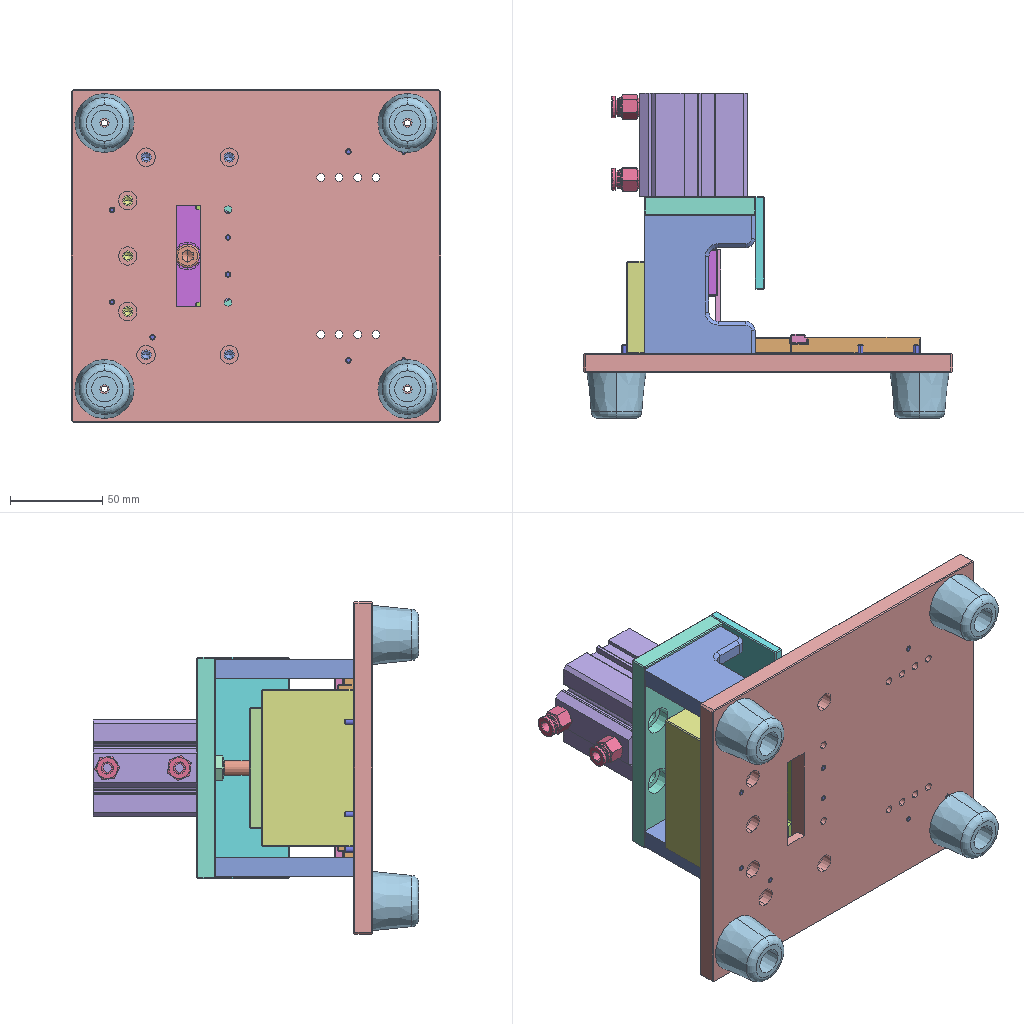Assembly | SolidWorks | 21 different items | 35 placed | box 200 x 176 x 180 mm
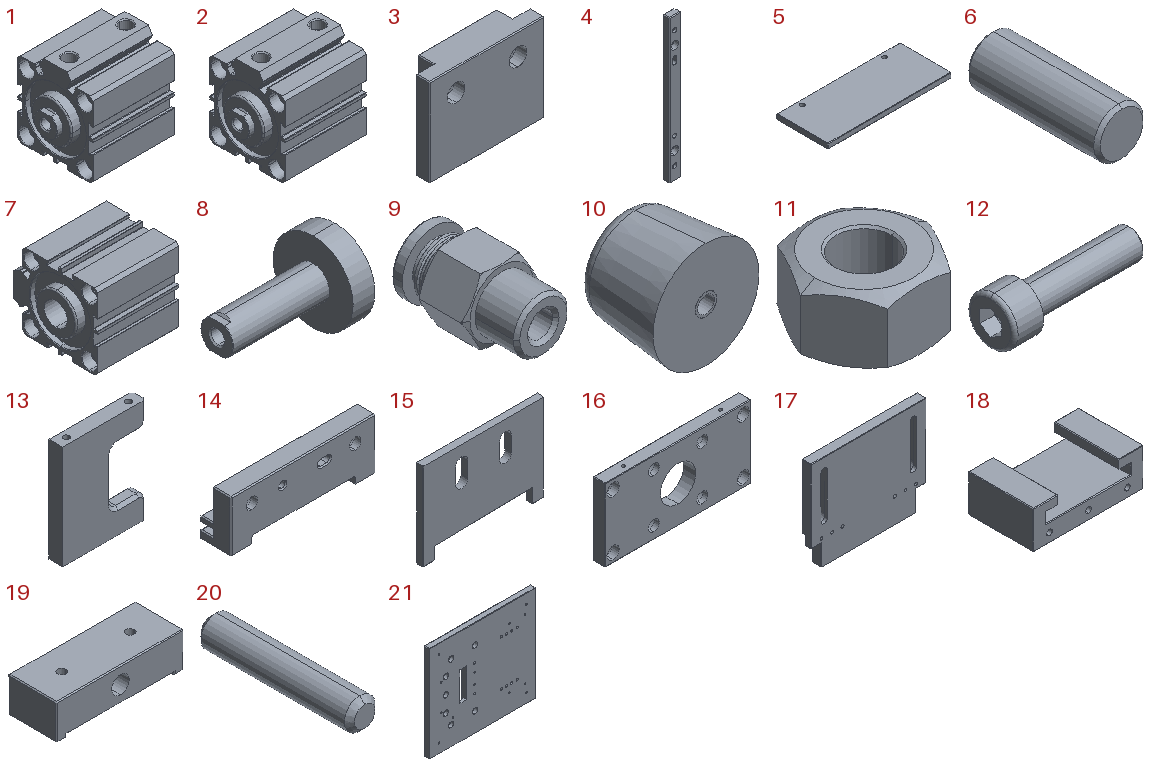Parts list (item | name | quantity | parent item | size | volume | features):
1 | (subassembly) | x1 | - | 63 x 52 x 58.5 mm | 102048 mm3 | -
2 | (subassembly) | x1 | in 1 | 63 x 52 x 58.5 mm | 102048 mm3 | -
3 | - | x1 | - | 65 x 18 x 50 mm | 45832 mm3 | features Chamfer 1, Extrusion 1, HoleWzd 1, ICE 1
4 | - | x1 | - | 9 x 5 x 110 mm | 4152 mm3 | features HoleWzd 3, Chamfer 1, Extrusion 1, ICE 1
5 | - | x1 | - | 120 x 50 x 5 mm | 29788 mm3 | features Chamfer 1, Extrusion 1, HoleWzd 1
6 | - | x2 | - | 3 x 8 x 3 mm | 56.188 mm3 | features Chamfer 1, Extrusion 1
7 | - | x1 | in 2 | 59 x 58.5 x 52 mm | 79787 mm3 | features MBimport 1
8 | - | x1 | in 2 | 58.5 x 39.5 x 39.5 mm | 22261 mm3 | features MBimport 1
9 | - | x2 | - | 13.856 x 21.5 x 12 mm | 1497 mm3 | features MBimport 1
10 | - | x4 | - | 32 x 25 x 32 mm | 14674 mm3 | features MBimport 1
11 | - | x1 | - | 15.011 x 13 x 7.5 mm | 813.544 mm3 | features RevCut 4, Chamfer 2, Boss 1, Extrusion 1, LPattern 1
12 | - | x1 | - | 38 x 13 x 13 mm | 2418 mm3 | features Fillet 2, RevCut 2, Boss 1, Chamfer 1, Cut 1, Extrusion 1, LPattern 1
13 | - | x2 | - | 60 x 10 x 75 mm | 33824 mm3 | features HoleWzd 2, Chamfer 1, Extrusion 1, Fillet 1, ICE 1
14 | - | x1 | - | 70 x 15 x 25 mm | 14234 mm3 | features Chamfer 5, ICE 3, Extrusion 1, Fillet 1, HoleWzd 1
15 | - | x1 | - | 55 x 3 x 40 mm | 5559 mm3 | features Chamfer 4, Draft 1, Extrusion 1, ICE 1
16 | - | x1 | - | 120 x 10 x 60 mm | 57722 mm3 | features HoleWzd 3, ICE 2, Chamfer 1, Extrusion 1
17 | - | x1 | - | 110 x 9 x 90 mm | 72991 mm3 | features ICE 6, Chamfer 3, HoleWzd 2, Extrusion 1, MoveFace 1
18 | - | x1 | - | 85 x 50 x 29 mm | 80145 mm3 | features Chamfer 2, Extrusion 1, HoleWzd 1, ICE 1, MoveFace 1
19 | - | x1 | - | 65 x 25 x 18 mm | 24148 mm3 | features Chamfer 4, HoleWzd 3, Extrusion 1, ICE 1
20 | - | x9 | - | 3 x 15 x 3 mm | 103.934 mm3 | features Chamfer 1, Extrusion 1
21 | - | x1 | - | 200 x 10 x 180 mm | 345218 mm3 | features HoleWzd 6, Chamfer 3, ICE 2, Extrusion 1
Mates (type | each side: item.copy, entity, surface, feature):
Concentric | 21.1 edge | 13.1 edge | 2 times
Coincident | 21.1 face plane Boss-Extrude1 | 13.1 face plane Boss-Extrude1
Coincident | 21.1 face plane Boss-Extrude1 | 14.1 face plane Boss-Extrude1
Width | 21.1 face plane Boss-Extrude1 | 21.1 face plane Boss-Extrude1 | 14.1 face plane Boss-Extrude1 | 14.1 face plane Boss-Extrude1
Concentric | 13.1 edge | 16.1 edge
Coincident | 13.1 face plane Boss-Extrude1 | 16.1 face plane Boss-Extrude1
Coincident | 21.1 face plane Boss-Extrude1 | 17.1 face plane Boss-Extrude1
Width | 17.1 face plane Cut-Extrude3 | 17.1 face plane Cut-Extrude3 | 14.1 face plane Boss-Extrude1 | 14.1 face plane Boss-Extrude1
LimitDistanceDim | 14.1 face plane Boss-Extrude1 | 17.1 face plane Boss-Extrude1
Concentric | 21.1 edge | 14.1 edge | 2 times
Concentric | 16.1 face cylinder CBORE for M8 Slotted cheese head screws1 | 7.1 face cylinder SDA40x30(0)+().stp<1> | 2 times
Coincident | 16.1 face plane Boss-Extrude1 | 7.1 face plane SDA40x30(0)+().stp<1>
Concentric | 7.1 face cylinder SDA40x30(0)+().stp<1> | 9.1 face cylinder BPC601.stp<1>
DistanceDim | 9.1 face plane BPC601.stp<1> | 7.1 face plane SDA40x30(0)+().stp<1>
Concentric | 7.1 face cylinder SDA40x30(0)+().stp<1> | 9.2 face cylinder BPC601.stp<1>
DistanceDim | 7.1 face plane SDA40x30(0)+().stp<1> | 9.2 face plane BPC601.stp<1>
Concentric | 10.1 face cylinder ECRKC3225.stp<1> | 21.1 face cylinder M4 Tapped Hole1
Coincident | 21.1 face plane Boss-Extrude1 | 10.1 face plane ECRKC3225.stp<1>
Concentric | 21.1 face cylinder M4 Tapped Hole1 | 10.2 face cylinder ECRKC3225.stp<1>
Coincident | 21.1 face plane Boss-Extrude1 | 10.2 face plane ECRKC3225.stp<1>
Concentric | 21.1 face cylinder M4 Tapped Hole1 | 10.3 face cylinder ECRKC3225.stp<1>
Coincident | 21.1 face plane Boss-Extrude1 | 10.3 face plane ECRKC3225.stp<1>
Concentric | 21.1 face cylinder M4 Tapped Hole1 | 10.4 face cylinder ECRKC3225.stp<1>
Coincident | 21.1 face plane Boss-Extrude1 | 10.4 face plane ECRKC3225.stp<1>
Coincident | 21.1 face plane Boss-Extrude1 | 18.1 face plane Boss-Extrude1
Concentric | 8.1 face cylinder SDA40x30(0)+().stp<1> | 11.1 face cylinder BaseNut
Coincident | 8.1 face plane SDA40x30(0)+().stp<1> | 11.1 face plane BaseNut
Concentric | 8.1 face cylinder SDA40x30(0)+().stp<1> | 12.1 face cylinder BaseBody
Concentric | 21.1 face cylinder Ø3.0mm dowel hole1 | 20.1 face cylinder Boss-Extrude1
Coincident | 21.1 face plane Boss-Extrude1 | 20.1 face plane Boss-Extrude1
Concentric | 21.1 face cylinder Ø3.0mm dowel hole1 | 20.2 face cylinder Boss-Extrude1
Coincident | 21.1 face plane Boss-Extrude1 | 20.2 face plane Boss-Extrude1
Concentric | 21.1 face cylinder Ø3.0mm dowel hole1 | 20.3 face cylinder Boss-Extrude1
Coincident | 21.1 face plane Boss-Extrude1 | 20.3 edge
Concentric | 21.1 face cylinder Cut-Extrude2 | 20.4 face cylinder Boss-Extrude1
Coincident | 21.1 face plane Boss-Extrude1 | 20.4 face plane Boss-Extrude1
Concentric | 21.1 face cylinder Cut-Extrude2 | 20.5 face cylinder Boss-Extrude1
Coincident | 21.1 face plane Boss-Extrude1 | 20.5 face plane Boss-Extrude1
Coincident | 19.1 face plane Boss-Extrude1 | 3.1 face plane Cut-Extrude1
Width | 3.1 face plane Boss-Extrude1 | 3.1 face plane Boss-Extrude1 | 18.1 face plane Cut-Extrude3 | 18.1 face plane Cut-Extrude3
Coincident | 18.1 face plane Cut-Extrude3 | 3.1 face plane Boss-Extrude1
LimitDistanceDim | 3.1 face plane Boss-Extrude1 | 21.1 face plane Boss-Extrude1
Width | 15.1 face plane Boss-Extrude1 | 15.1 face plane Boss-Extrude1 | 19.1 face plane Boss-Extrude1 | 19.1 face plane Boss-Extrude1
Coincident | 15.1 face plane Boss-Extrude1 | 19.1 face plane Boss-Extrude1 | 2 times
Coincident | 19.1 face plane CBORE for M8 Slotted cheese head screws1 | 12.1 face plane BaseHead
Concentric | 21.1 face cylinder CBORE for M5 Slotted cheese head screws2 | 18.1 face cylinder M5 Tapped Hole1 | 2 times
Concentric | 19.1 face cylinder M5 Tapped Hole2 | 3.1 face cylinder CBORE for M5 Slotted cheese head screws1 | 2 times
Concentric | 21.1 face cylinder CBORE for M5 Slotted cheese head screws1 | 13.2 face cylinder M5 Tapped Hole1 | 2 times
Coincident | 21.1 face plane Boss-Extrude1 | 13.2 face plane Boss-Extrude1
Concentric | 16.1 face cylinder CBORE for M5 Slotted cheese head screws1 | 13.2 face cylinder M5 Tapped Hole2
Concentric | 16.1 face cylinder M3 Tapped Hole1 | 5.1 face cylinder Ø4.0mm dowel hole1 | 2 times
Coincident | 16.1 face plane Boss-Extrude1 | 5.1 face plane Boss-Extrude1
Coincident | 17.1 face plane Cut-Extrude5 | 4.1 face plane Boss-Extrude2
Concentric | 17.1 face cylinder M3 Tapped Hole1 | 4.1 face cylinder CBORE for M3 Slotted cheese head screws2 | 2 times
Concentric | 21.1 face cylinder Ø3.0mm dowel hole2 | 20.6 face cylinder Boss-Extrude1
Coincident | 21.1 face plane Boss-Extrude1 | 20.6 face plane Boss-Extrude1
Concentric | 21.1 face cylinder Ø3.0mm dowel hole2 | 20.7 face cylinder Boss-Extrude1
Coincident | 21.1 face plane Boss-Extrude1 | 20.7 face plane Boss-Extrude1
Concentric | 17.1 face cylinder Ø3.0mm dowel hole1 | 6.1 face cylinder Boss-Extrude1
Coincident | 17.1 face plane Boss-Extrude1 | 6.1 face plane Boss-Extrude1